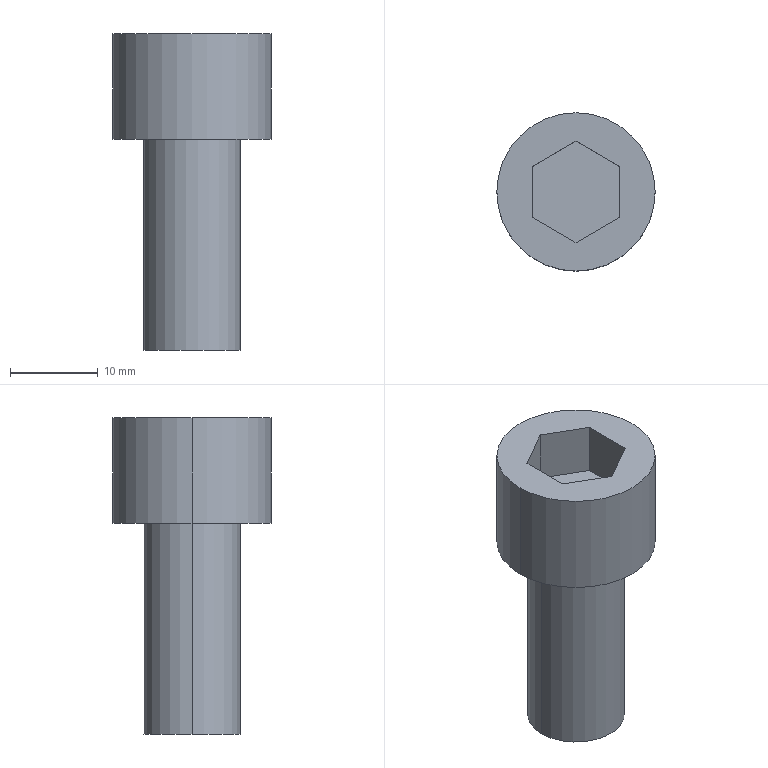Part | SolidWorks | features ICE 2, Extrusion 1 | 1 solid | 14 faces | box 18 x 18 x 36 mm | volume 4815 mm3 | plane 10 | cylinder 4 | commonest cylinder face diameters 11 x2 18 x2
STEP:
#1=CARTESIAN_POINT('',(9.,0.,36.));
#2=VERTEX_POINT('',#1);
#3=CARTESIAN_POINT('',(-9.,0.,36.));
#4=VERTEX_POINT('',#3);
#5=CARTESIAN_POINT('',(0.,0.,36.));
#6=DIRECTION('',(0.,0.,1.));
#7=DIRECTION('',(1.,0.,0.));
#8=AXIS2_PLACEMENT_3D('',#5,#6,#7);
#9=CIRCLE('',#8,9.);
#10=EDGE_CURVE('',#2,#4,#9,.T.);
#11=ORIENTED_EDGE('',*,*,#10,.F.);
#12=CARTESIAN_POINT('',(9.,0.,24.));
#13=VERTEX_POINT('',#12);
#14=CARTESIAN_POINT('',(9.,0.,36.));
#15=DIRECTION('',(0.,0.,-1.));
#16=VECTOR('',#15,1000.);
#17=LINE('',#14,#16);
#18=EDGE_CURVE('',#2,#13,#17,.T.);
#19=ORIENTED_EDGE('',*,*,#18,.T.);
#20=CARTESIAN_POINT('',(-9.,0.,24.));
#21=VERTEX_POINT('',#20);
#22=CARTESIAN_POINT('',(0.,0.,24.));
#23=DIRECTION('',(0.,0.,1.));
#24=DIRECTION('',(1.,0.,0.));
#25=AXIS2_PLACEMENT_3D('',#22,#23,#24);
#26=CIRCLE('',#25,9.);
#27=EDGE_CURVE('',#13,#21,#26,.T.);
#28=ORIENTED_EDGE('',*,*,#27,.T.);
#29=CARTESIAN_POINT('',(-9.,0.,36.));
#30=DIRECTION('',(0.,0.,-1.));
#31=VECTOR('',#30,1000.);
#32=LINE('',#29,#31);
#33=EDGE_CURVE('',#4,#21,#32,.T.);
#34=ORIENTED_EDGE('',*,*,#33,.F.);
#35=EDGE_LOOP('',(#11,#19,#28,#34));
#36=FACE_OUTER_BOUND('',#35,.T.);
#37=CARTESIAN_POINT('',(0.,0.,36.));
#38=DIRECTION('',(0.,0.,-1.));
#39=DIRECTION('',(-1.,0.,0.));
#40=AXIS2_PLACEMENT_3D('',#37,#38,#39);
#41=CYLINDRICAL_SURFACE('',#40,9.);
#42=ADVANCED_FACE('',(#36),#41,.T.);
#43=CARTESIAN_POINT('',(5.5,0.,24.));
#44=VERTEX_POINT('',#43);
#45=CARTESIAN_POINT('',(-5.5,0.,24.));
#46=VERTEX_POINT('',#45);
#47=CARTESIAN_POINT('',(0.,0.,24.));
#48=DIRECTION('',(0.,0.,1.));
#49=DIRECTION('',(1.,0.,0.));
#50=AXIS2_PLACEMENT_3D('',#47,#48,#49);
#51=CIRCLE('',#50,5.5);
#52=EDGE_CURVE('',#44,#46,#51,.T.);
#53=ORIENTED_EDGE('',*,*,#52,.F.);
#54=CARTESIAN_POINT('',(5.5,0.,0.));
#55=VERTEX_POINT('',#54);
#56=CARTESIAN_POINT('',(5.5,0.,24.));
#57=DIRECTION('',(0.,0.,-1.));
#58=VECTOR('',#57,1000.);
#59=LINE('',#56,#58);
#60=EDGE_CURVE('',#44,#55,#59,.T.);
#61=ORIENTED_EDGE('',*,*,#60,.T.);
#62=CARTESIAN_POINT('',(-5.5,0.,0.));
#63=VERTEX_POINT('',#62);
#64=CARTESIAN_POINT('',(0.,0.,0.));
#65=DIRECTION('',(0.,0.,1.));
#66=DIRECTION('',(1.,0.,0.));
#67=AXIS2_PLACEMENT_3D('',#64,#65,#66);
#68=CIRCLE('',#67,5.5);
#69=EDGE_CURVE('',#55,#63,#68,.T.);
#70=ORIENTED_EDGE('',*,*,#69,.T.);
#71=CARTESIAN_POINT('',(-5.5,0.,24.));
#72=DIRECTION('',(0.,0.,-1.));
#73=VECTOR('',#72,1000.);
#74=LINE('',#71,#73);
#75=EDGE_CURVE('',#46,#63,#74,.T.);
#76=ORIENTED_EDGE('',*,*,#75,.F.);
#77=EDGE_LOOP('',(#53,#61,#70,#76));
#78=FACE_OUTER_BOUND('',#77,.T.);
#79=CARTESIAN_POINT('',(0.,0.,24.));
#80=DIRECTION('',(0.,0.,-1.));
#81=DIRECTION('',(-1.,0.,0.));
#82=AXIS2_PLACEMENT_3D('',#79,#80,#81);
#83=CYLINDRICAL_SURFACE('',#82,5.5);
#84=ADVANCED_FACE('',(#78),#83,.T.);
#85=ORIENTED_EDGE('',*,*,#60,.F.);
#86=CARTESIAN_POINT('',(0.,0.,24.));
#87=DIRECTION('',(0.,0.,1.));
#88=DIRECTION('',(1.,0.,0.));
#89=AXIS2_PLACEMENT_3D('',#86,#87,#88);
#90=CIRCLE('',#89,5.5);
#91=EDGE_CURVE('',#46,#44,#90,.T.);
#92=ORIENTED_EDGE('',*,*,#91,.F.);
#93=ORIENTED_EDGE('',*,*,#75,.T.);
#94=CARTESIAN_POINT('',(0.,0.,0.));
#95=DIRECTION('',(0.,0.,1.));
#96=DIRECTION('',(1.,0.,0.));
#97=AXIS2_PLACEMENT_3D('',#94,#95,#96);
#98=CIRCLE('',#97,5.5);
#99=EDGE_CURVE('',#63,#55,#98,.T.);
#100=ORIENTED_EDGE('',*,*,#99,.T.);
#101=EDGE_LOOP('',(#85,#92,#93,#100));
#102=FACE_OUTER_BOUND('',#101,.T.);
#103=CARTESIAN_POINT('',(0.,0.,24.));
#104=DIRECTION('',(0.,0.,-1.));
#105=DIRECTION('',(-1.,0.,0.));
#106=AXIS2_PLACEMENT_3D('',#103,#104,#105);
#107=CYLINDRICAL_SURFACE('',#106,5.5);
#108=ADVANCED_FACE('',(#102),#107,.T.);
#109=ORIENTED_EDGE('',*,*,#99,.F.);
#110=ORIENTED_EDGE('',*,*,#69,.F.);
#111=EDGE_LOOP('',(#109,#110));
#112=FACE_OUTER_BOUND('',#111,.T.);
#113=CARTESIAN_POINT('',(0.,0.,0.));
#114=DIRECTION('',(0.,0.,1.));
#115=DIRECTION('',(1.,0.,0.));
#116=AXIS2_PLACEMENT_3D('',#113,#114,#115);
#117=PLANE('',#116);
#118=ADVANCED_FACE('',(#112),#117,.F.);
#119=CARTESIAN_POINT('',(0.,0.,24.));
#120=DIRECTION('',(0.,0.,1.));
#121=DIRECTION('',(1.,0.,0.));
#122=AXIS2_PLACEMENT_3D('',#119,#120,#121);
#123=CIRCLE('',#122,9.);
#124=EDGE_CURVE('',#21,#13,#123,.T.);
#125=ORIENTED_EDGE('',*,*,#124,.F.);
#126=ORIENTED_EDGE('',*,*,#27,.F.);
#127=EDGE_LOOP('',(#125,#126));
#128=FACE_OUTER_BOUND('',#127,.T.);
#129=ORIENTED_EDGE('',*,*,#91,.T.);
#130=ORIENTED_EDGE('',*,*,#52,.T.);
#131=EDGE_LOOP('',(#129,#130));
#132=FACE_BOUND('',#131,.T.);
#133=CARTESIAN_POINT('',(0.,0.,24.));
#134=DIRECTION('',(0.,0.,1.));
#135=DIRECTION('',(1.,0.,0.));
#136=AXIS2_PLACEMENT_3D('',#133,#134,#135);
#137=PLANE('',#136);
#138=ADVANCED_FACE('',(#128,#132),#137,.F.);
#139=ORIENTED_EDGE('',*,*,#18,.F.);
#140=CARTESIAN_POINT('',(0.,0.,36.));
#141=DIRECTION('',(0.,0.,1.));
#142=DIRECTION('',(1.,0.,0.));
#143=AXIS2_PLACEMENT_3D('',#140,#141,#142);
#144=CIRCLE('',#143,9.);
#145=EDGE_CURVE('',#4,#2,#144,.T.);
#146=ORIENTED_EDGE('',*,*,#145,.F.);
#147=ORIENTED_EDGE('',*,*,#33,.T.);
#148=ORIENTED_EDGE('',*,*,#124,.T.);
#149=EDGE_LOOP('',(#139,#146,#147,#148));
#150=FACE_OUTER_BOUND('',#149,.T.);
#151=CARTESIAN_POINT('',(0.,0.,36.));
#152=DIRECTION('',(0.,0.,-1.));
#153=DIRECTION('',(-1.,0.,0.));
#154=AXIS2_PLACEMENT_3D('',#151,#152,#153);
#155=CYLINDRICAL_SURFACE('',#154,9.);
#156=ADVANCED_FACE('',(#150),#155,.T.);
#157=CARTESIAN_POINT('',(5.,2.887,36.));
#158=VERTEX_POINT('',#157);
#159=CARTESIAN_POINT('',(0.,5.774,36.));
#160=VERTEX_POINT('',#159);
#161=CARTESIAN_POINT('',(5.,2.887,36.));
#162=DIRECTION('',(-0.866,0.5,0.));
#163=VECTOR('',#162,1000.);
#164=LINE('',#161,#163);
#165=EDGE_CURVE('',#158,#160,#164,.T.);
#166=ORIENTED_EDGE('',*,*,#165,.F.);
#167=CARTESIAN_POINT('',(5.,-2.887,36.));
#168=VERTEX_POINT('',#167);
#169=CARTESIAN_POINT('',(5.,-2.887,36.));
#170=DIRECTION('',(0.,1.,0.));
#171=VECTOR('',#170,1000.);
#172=LINE('',#169,#171);
#173=EDGE_CURVE('',#168,#158,#172,.T.);
#174=ORIENTED_EDGE('',*,*,#173,.F.);
#175=CARTESIAN_POINT('',(0.,-5.774,36.));
#176=VERTEX_POINT('',#175);
#177=CARTESIAN_POINT('',(0.,-5.774,36.));
#178=DIRECTION('',(0.866,0.5,0.));
#179=VECTOR('',#178,1000.);
#180=LINE('',#177,#179);
#181=EDGE_CURVE('',#176,#168,#180,.T.);
#182=ORIENTED_EDGE('',*,*,#181,.F.);
#183=CARTESIAN_POINT('',(-5.,-2.887,36.));
#184=VERTEX_POINT('',#183);
#185=CARTESIAN_POINT('',(-5.,-2.887,36.));
#186=DIRECTION('',(0.866,-0.5,0.));
#187=VECTOR('',#186,1000.);
#188=LINE('',#185,#187);
#189=EDGE_CURVE('',#184,#176,#188,.T.);
#190=ORIENTED_EDGE('',*,*,#189,.F.);
#191=CARTESIAN_POINT('',(-5.,2.887,36.));
#192=VERTEX_POINT('',#191);
#193=CARTESIAN_POINT('',(-5.,2.887,36.));
#194=DIRECTION('',(0.,-1.,0.));
#195=VECTOR('',#194,1000.);
#196=LINE('',#193,#195);
#197=EDGE_CURVE('',#192,#184,#196,.T.);
#198=ORIENTED_EDGE('',*,*,#197,.F.);
#199=CARTESIAN_POINT('',(0.,5.774,36.));
#200=DIRECTION('',(-0.866,-0.5,0.));
#201=VECTOR('',#200,1000.);
#202=LINE('',#199,#201);
#203=EDGE_CURVE('',#160,#192,#202,.T.);
#204=ORIENTED_EDGE('',*,*,#203,.F.);
#205=EDGE_LOOP('',(#166,#174,#182,#190,#198,#204));
#206=FACE_BOUND('',#205,.T.);
#207=ORIENTED_EDGE('',*,*,#145,.T.);
#208=ORIENTED_EDGE('',*,*,#10,.T.);
#209=EDGE_LOOP('',(#207,#208));
#210=FACE_OUTER_BOUND('',#209,.T.);
#211=CARTESIAN_POINT('',(0.,0.,36.));
#212=DIRECTION('',(0.,0.,1.));
#213=DIRECTION('',(1.,0.,0.));
#214=AXIS2_PLACEMENT_3D('',#211,#212,#213);
#215=PLANE('',#214);
#216=ADVANCED_FACE('',(#206,#210),#215,.T.);
#217=ORIENTED_EDGE('',*,*,#165,.T.);
#218=CARTESIAN_POINT('',(0.,5.774,30.));
#219=VERTEX_POINT('',#218);
#220=CARTESIAN_POINT('',(0.,5.774,30.));
#221=DIRECTION('',(0.,0.,1.));
#222=VECTOR('',#221,1000.);
#223=LINE('',#220,#222);
#224=EDGE_CURVE('',#219,#160,#223,.T.);
#225=ORIENTED_EDGE('',*,*,#224,.F.);
#226=CARTESIAN_POINT('',(5.,2.887,30.));
#227=VERTEX_POINT('',#226);
#228=CARTESIAN_POINT('',(5.,2.887,30.));
#229=DIRECTION('',(-0.866,0.5,0.));
#230=VECTOR('',#229,1000.);
#231=LINE('',#228,#230);
#232=EDGE_CURVE('',#227,#219,#231,.T.);
#233=ORIENTED_EDGE('',*,*,#232,.F.);
#234=CARTESIAN_POINT('',(5.,2.887,30.));
#235=DIRECTION('',(0.,0.,1.));
#236=VECTOR('',#235,1000.);
#237=LINE('',#234,#236);
#238=EDGE_CURVE('',#227,#158,#237,.T.);
#239=ORIENTED_EDGE('',*,*,#238,.T.);
#240=EDGE_LOOP('',(#217,#225,#233,#239));
#241=FACE_OUTER_BOUND('',#240,.T.);
#242=CARTESIAN_POINT('',(5.,2.887,30.));
#243=DIRECTION('',(0.5,0.866,0.));
#244=DIRECTION('',(-0.866,0.5,0.));
#245=AXIS2_PLACEMENT_3D('',#242,#243,#244);
#246=PLANE('',#245);
#247=ADVANCED_FACE('',(#241),#246,.F.);
#248=ORIENTED_EDGE('',*,*,#173,.T.);
#249=ORIENTED_EDGE('',*,*,#238,.F.);
#250=CARTESIAN_POINT('',(5.,-2.887,30.));
#251=VERTEX_POINT('',#250);
#252=CARTESIAN_POINT('',(5.,-2.887,30.));
#253=DIRECTION('',(0.,1.,0.));
#254=VECTOR('',#253,1000.);
#255=LINE('',#252,#254);
#256=EDGE_CURVE('',#251,#227,#255,.T.);
#257=ORIENTED_EDGE('',*,*,#256,.F.);
#258=CARTESIAN_POINT('',(5.,-2.887,30.));
#259=DIRECTION('',(0.,0.,1.));
#260=VECTOR('',#259,1000.);
#261=LINE('',#258,#260);
#262=EDGE_CURVE('',#251,#168,#261,.T.);
#263=ORIENTED_EDGE('',*,*,#262,.T.);
#264=EDGE_LOOP('',(#248,#249,#257,#263));
#265=FACE_OUTER_BOUND('',#264,.T.);
#266=CARTESIAN_POINT('',(5.,-2.887,30.));
#267=DIRECTION('',(1.,0.,0.));
#268=DIRECTION('',(0.,1.,0.));
#269=AXIS2_PLACEMENT_3D('',#266,#267,#268);
#270=PLANE('',#269);
#271=ADVANCED_FACE('',(#265),#270,.F.);
#272=ORIENTED_EDGE('',*,*,#181,.T.);
#273=ORIENTED_EDGE('',*,*,#262,.F.);
#274=CARTESIAN_POINT('',(0.,-5.774,30.));
#275=VERTEX_POINT('',#274);
#276=CARTESIAN_POINT('',(0.,-5.774,30.));
#277=DIRECTION('',(0.866,0.5,0.));
#278=VECTOR('',#277,1000.);
#279=LINE('',#276,#278);
#280=EDGE_CURVE('',#275,#251,#279,.T.);
#281=ORIENTED_EDGE('',*,*,#280,.F.);
#282=CARTESIAN_POINT('',(0.,-5.774,30.));
#283=DIRECTION('',(0.,0.,1.));
#284=VECTOR('',#283,1000.);
#285=LINE('',#282,#284);
#286=EDGE_CURVE('',#275,#176,#285,.T.);
#287=ORIENTED_EDGE('',*,*,#286,.T.);
#288=EDGE_LOOP('',(#272,#273,#281,#287));
#289=FACE_OUTER_BOUND('',#288,.T.);
#290=CARTESIAN_POINT('',(0.,-5.774,30.));
#291=DIRECTION('',(0.5,-0.866,0.));
#292=DIRECTION('',(0.866,0.5,0.));
#293=AXIS2_PLACEMENT_3D('',#290,#291,#292);
#294=PLANE('',#293);
#295=ADVANCED_FACE('',(#289),#294,.F.);
#296=ORIENTED_EDGE('',*,*,#189,.T.);
#297=ORIENTED_EDGE('',*,*,#286,.F.);
#298=CARTESIAN_POINT('',(-5.,-2.887,30.));
#299=VERTEX_POINT('',#298);
#300=CARTESIAN_POINT('',(-5.,-2.887,30.));
#301=DIRECTION('',(0.866,-0.5,0.));
#302=VECTOR('',#301,1000.);
#303=LINE('',#300,#302);
#304=EDGE_CURVE('',#299,#275,#303,.T.);
#305=ORIENTED_EDGE('',*,*,#304,.F.);
#306=CARTESIAN_POINT('',(-5.,-2.887,30.));
#307=DIRECTION('',(0.,0.,1.));
#308=VECTOR('',#307,1000.);
#309=LINE('',#306,#308);
#310=EDGE_CURVE('',#299,#184,#309,.T.);
#311=ORIENTED_EDGE('',*,*,#310,.T.);
#312=EDGE_LOOP('',(#296,#297,#305,#311));
#313=FACE_OUTER_BOUND('',#312,.T.);
#314=CARTESIAN_POINT('',(-5.,-2.887,30.));
#315=DIRECTION('',(-0.5,-0.866,0.));
#316=DIRECTION('',(0.866,-0.5,0.));
#317=AXIS2_PLACEMENT_3D('',#314,#315,#316);
#318=PLANE('',#317);
#319=ADVANCED_FACE('',(#313),#318,.F.);
#320=ORIENTED_EDGE('',*,*,#197,.T.);
#321=ORIENTED_EDGE('',*,*,#310,.F.);
#322=CARTESIAN_POINT('',(-5.,2.887,30.));
#323=VERTEX_POINT('',#322);
#324=CARTESIAN_POINT('',(-5.,2.887,30.));
#325=DIRECTION('',(0.,-1.,0.));
#326=VECTOR('',#325,1000.);
#327=LINE('',#324,#326);
#328=EDGE_CURVE('',#323,#299,#327,.T.);
#329=ORIENTED_EDGE('',*,*,#328,.F.);
#330=CARTESIAN_POINT('',(-5.,2.887,30.));
#331=DIRECTION('',(0.,0.,1.));
#332=VECTOR('',#331,1000.);
#333=LINE('',#330,#332);
#334=EDGE_CURVE('',#323,#192,#333,.T.);
#335=ORIENTED_EDGE('',*,*,#334,.T.);
#336=EDGE_LOOP('',(#320,#321,#329,#335));
#337=FACE_OUTER_BOUND('',#336,.T.);
#338=CARTESIAN_POINT('',(-5.,2.887,30.));
#339=DIRECTION('',(-1.,0.,0.));
#340=DIRECTION('',(0.,0.,1.));
#341=AXIS2_PLACEMENT_3D('',#338,#339,#340);
#342=PLANE('',#341);
#343=ADVANCED_FACE('',(#337),#342,.F.);
#344=ORIENTED_EDGE('',*,*,#203,.T.);
#345=ORIENTED_EDGE('',*,*,#334,.F.);
#346=CARTESIAN_POINT('',(0.,5.774,30.));
#347=DIRECTION('',(-0.866,-0.5,0.));
#348=VECTOR('',#347,1000.);
#349=LINE('',#346,#348);
#350=EDGE_CURVE('',#219,#323,#349,.T.);
#351=ORIENTED_EDGE('',*,*,#350,.F.);
#352=ORIENTED_EDGE('',*,*,#224,.T.);
#353=EDGE_LOOP('',(#344,#345,#351,#352));
#354=FACE_OUTER_BOUND('',#353,.T.);
#355=CARTESIAN_POINT('',(0.,5.774,30.));
#356=DIRECTION('',(-0.5,0.866,0.));
#357=DIRECTION('',(-0.866,-0.5,0.));
#358=AXIS2_PLACEMENT_3D('',#355,#356,#357);
#359=PLANE('',#358);
#360=ADVANCED_FACE('',(#354),#359,.F.);
#361=ORIENTED_EDGE('',*,*,#232,.T.);
#362=ORIENTED_EDGE('',*,*,#350,.T.);
#363=ORIENTED_EDGE('',*,*,#328,.T.);
#364=ORIENTED_EDGE('',*,*,#304,.T.);
#365=ORIENTED_EDGE('',*,*,#280,.T.);
#366=ORIENTED_EDGE('',*,*,#256,.T.);
#367=EDGE_LOOP('',(#361,#362,#363,#364,#365,#366));
#368=FACE_OUTER_BOUND('',#367,.T.);
#369=CARTESIAN_POINT('',(0.,0.,30.));
#370=DIRECTION('',(0.,0.,1.));
#371=DIRECTION('',(1.,0.,0.));
#372=AXIS2_PLACEMENT_3D('',#369,#370,#371);
#373=PLANE('',#372);
#374=ADVANCED_FACE('',(#368),#373,.T.);
#375=CLOSED_SHELL('',(#42,#84,#108,#118,#138,#156,#216,#247,#271,#295,#319,#343,#360,#374));
#376=MANIFOLD_SOLID_BREP('',#375);
#377=CARTESIAN_POINT('',(0.,0.,0.));
#378=DIRECTION('',(0.,0.,1.));
#379=DIRECTION('',(1.,0.,0.));
#380=AXIS2_PLACEMENT_3D('',#377,#378,#379);
#381=(LENGTH_UNIT()NAMED_UNIT(*)SI_UNIT(.MILLI.,.METRE.));
#382=UNCERTAINTY_MEASURE_WITH_UNIT(LENGTH_MEASURE(0.00001),#381,'','');
#383=(NAMED_UNIT(*)PLANE_ANGLE_UNIT()SI_UNIT($,.RADIAN.));
#384=(NAMED_UNIT(*)SI_UNIT($,.STERADIAN.)SOLID_ANGLE_UNIT());
#385=(GEOMETRIC_REPRESENTATION_CONTEXT(3)GLOBAL_UNCERTAINTY_ASSIGNED_CONTEXT((#382))GLOBAL_UNIT_ASSIGNED_CONTEXT((#381,#383,#384))REPRESENTATION_CONTEXT('',''));
#386=ADVANCED_BREP_SHAPE_REPRESENTATION('',(#376,#380),#385);